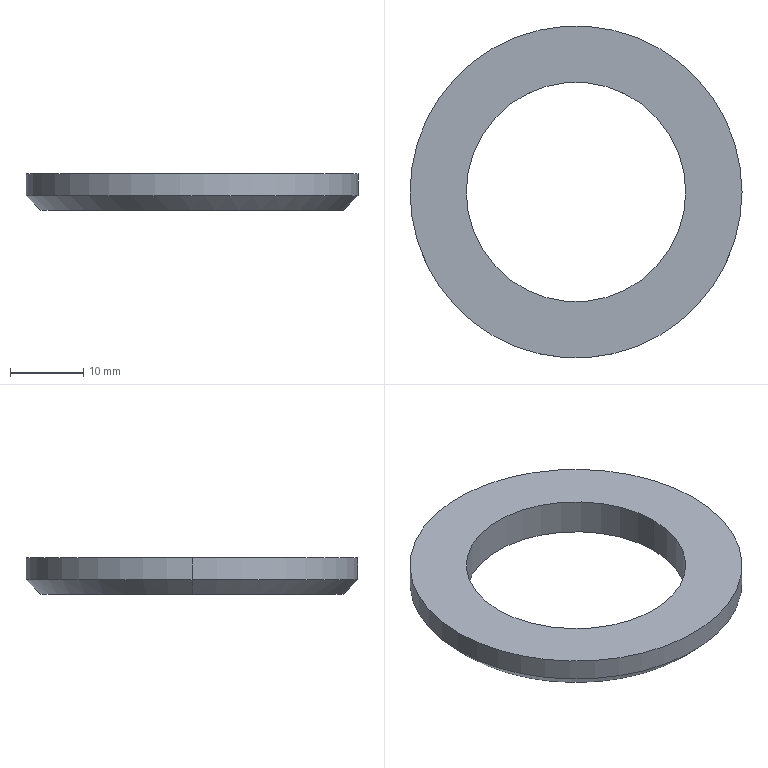Part | SolidWorks | features Chamfer 1, Extrusion 1 | 1 solid | 8 faces | box 45.387 x 45.387 x 5 mm | volume 4279 mm3 | cylinder 4 | cone 2 | plane 2 | commonest cylinder face diameters 30 x2 45.387 x2
STEP:
#1=CARTESIAN_POINT('',(49.306,-13.,0.));
#2=VERTEX_POINT('',#1);
#3=CARTESIAN_POINT('',(90.694,-13.,0.));
#4=VERTEX_POINT('',#3);
#5=CARTESIAN_POINT('',(70.,-13.,0.));
#6=DIRECTION('',(0.,0.,-1.));
#7=DIRECTION('',(1.,0.,0.));
#8=AXIS2_PLACEMENT_3D('',#5,#6,#7);
#9=CIRCLE('',#8,20.694);
#10=EDGE_CURVE('',#2,#4,#9,.T.);
#11=ORIENTED_EDGE('',*,*,#10,.F.);
#12=CARTESIAN_POINT('',(47.306,-13.,2.));
#13=VERTEX_POINT('',#12);
#14=CARTESIAN_POINT('',(47.306,-13.,2.));
#15=DIRECTION('',(-0.7071,0.,0.7071));
#16=VECTOR('',#15,1000.);
#17=LINE('',#14,#16);
#18=EDGE_CURVE('',#2,#13,#17,.T.);
#19=ORIENTED_EDGE('',*,*,#18,.T.);
#20=CARTESIAN_POINT('',(92.694,-13.,2.));
#21=VERTEX_POINT('',#20);
#22=CARTESIAN_POINT('',(70.,-13.,2.));
#23=DIRECTION('',(0.,0.,1.));
#24=DIRECTION('',(1.,0.,0.));
#25=AXIS2_PLACEMENT_3D('',#22,#23,#24);
#26=CIRCLE('',#25,22.694);
#27=EDGE_CURVE('',#21,#13,#26,.T.);
#28=ORIENTED_EDGE('',*,*,#27,.F.);
#29=CARTESIAN_POINT('',(92.694,-13.,2.));
#30=DIRECTION('',(0.7071,0.,0.7071));
#31=VECTOR('',#30,1000.);
#32=LINE('',#29,#31);
#33=EDGE_CURVE('',#4,#21,#32,.T.);
#34=ORIENTED_EDGE('',*,*,#33,.F.);
#35=EDGE_LOOP('',(#11,#19,#28,#34));
#36=FACE_OUTER_BOUND('',#35,.T.);
#37=CARTESIAN_POINT('',(70.,-13.,2.));
#38=DIRECTION('',(0.,0.,1.));
#39=DIRECTION('',(1.,0.,0.));
#40=AXIS2_PLACEMENT_3D('',#37,#38,#39);
#41=CONICAL_SURFACE('',#40,22.694,0.7854);
#42=ADVANCED_FACE('',(#36),#41,.T.);
#43=CARTESIAN_POINT('',(55.,-13.,5.));
#44=VERTEX_POINT('',#43);
#45=CARTESIAN_POINT('',(85.,-13.,5.));
#46=VERTEX_POINT('',#45);
#47=CARTESIAN_POINT('',(70.,-13.,5.));
#48=DIRECTION('',(0.,0.,1.));
#49=DIRECTION('',(1.,0.,0.));
#50=AXIS2_PLACEMENT_3D('',#47,#48,#49);
#51=CIRCLE('',#50,15.);
#52=EDGE_CURVE('',#44,#46,#51,.T.);
#53=ORIENTED_EDGE('',*,*,#52,.T.);
#54=CARTESIAN_POINT('',(85.,-13.,0.));
#55=VERTEX_POINT('',#54);
#56=CARTESIAN_POINT('',(85.,-13.,5.));
#57=DIRECTION('',(0.,0.,-1.));
#58=VECTOR('',#57,1000.);
#59=LINE('',#56,#58);
#60=EDGE_CURVE('',#46,#55,#59,.T.);
#61=ORIENTED_EDGE('',*,*,#60,.T.);
#62=CARTESIAN_POINT('',(55.,-13.,0.));
#63=VERTEX_POINT('',#62);
#64=CARTESIAN_POINT('',(70.,-13.,0.));
#65=DIRECTION('',(0.,0.,1.));
#66=DIRECTION('',(1.,0.,0.));
#67=AXIS2_PLACEMENT_3D('',#64,#65,#66);
#68=CIRCLE('',#67,15.);
#69=EDGE_CURVE('',#63,#55,#68,.T.);
#70=ORIENTED_EDGE('',*,*,#69,.F.);
#71=CARTESIAN_POINT('',(55.,-13.,5.));
#72=DIRECTION('',(0.,0.,-1.));
#73=VECTOR('',#72,1000.);
#74=LINE('',#71,#73);
#75=EDGE_CURVE('',#44,#63,#74,.T.);
#76=ORIENTED_EDGE('',*,*,#75,.F.);
#77=EDGE_LOOP('',(#53,#61,#70,#76));
#78=FACE_OUTER_BOUND('',#77,.T.);
#79=CARTESIAN_POINT('',(70.,-13.,5.));
#80=DIRECTION('',(0.,0.,-1.));
#81=DIRECTION('',(-1.,0.,0.));
#82=AXIS2_PLACEMENT_3D('',#79,#80,#81);
#83=CYLINDRICAL_SURFACE('',#82,15.);
#84=ADVANCED_FACE('',(#78),#83,.F.);
#85=CARTESIAN_POINT('',(92.694,-13.,5.));
#86=VERTEX_POINT('',#85);
#87=CARTESIAN_POINT('',(47.306,-13.,5.));
#88=VERTEX_POINT('',#87);
#89=CARTESIAN_POINT('',(70.,-13.,5.));
#90=DIRECTION('',(0.,0.,1.));
#91=DIRECTION('',(1.,0.,0.));
#92=AXIS2_PLACEMENT_3D('',#89,#90,#91);
#93=CIRCLE('',#92,22.694);
#94=EDGE_CURVE('',#86,#88,#93,.T.);
#95=ORIENTED_EDGE('',*,*,#94,.F.);
#96=CARTESIAN_POINT('',(92.694,-13.,5.));
#97=DIRECTION('',(0.,0.,-1.));
#98=VECTOR('',#97,1000.);
#99=LINE('',#96,#98);
#100=EDGE_CURVE('',#86,#21,#99,.T.);
#101=ORIENTED_EDGE('',*,*,#100,.T.);
#102=ORIENTED_EDGE('',*,*,#27,.T.);
#103=CARTESIAN_POINT('',(47.306,-13.,5.));
#104=DIRECTION('',(0.,0.,-1.));
#105=VECTOR('',#104,1000.);
#106=LINE('',#103,#105);
#107=EDGE_CURVE('',#88,#13,#106,.T.);
#108=ORIENTED_EDGE('',*,*,#107,.F.);
#109=EDGE_LOOP('',(#95,#101,#102,#108));
#110=FACE_OUTER_BOUND('',#109,.T.);
#111=CARTESIAN_POINT('',(70.,-13.,5.));
#112=DIRECTION('',(0.,0.,-1.));
#113=DIRECTION('',(-1.,0.,0.));
#114=AXIS2_PLACEMENT_3D('',#111,#112,#113);
#115=CYLINDRICAL_SURFACE('',#114,22.694);
#116=ADVANCED_FACE('',(#110),#115,.T.);
#117=CARTESIAN_POINT('',(70.,-13.,5.));
#118=DIRECTION('',(0.,0.,1.));
#119=DIRECTION('',(1.,0.,0.));
#120=AXIS2_PLACEMENT_3D('',#117,#118,#119);
#121=CIRCLE('',#120,22.694);
#122=EDGE_CURVE('',#88,#86,#121,.T.);
#123=ORIENTED_EDGE('',*,*,#122,.T.);
#124=ORIENTED_EDGE('',*,*,#94,.T.);
#125=EDGE_LOOP('',(#123,#124));
#126=FACE_OUTER_BOUND('',#125,.T.);
#127=ORIENTED_EDGE('',*,*,#52,.F.);
#128=CARTESIAN_POINT('',(70.,-13.,5.));
#129=DIRECTION('',(0.,0.,1.));
#130=DIRECTION('',(1.,0.,0.));
#131=AXIS2_PLACEMENT_3D('',#128,#129,#130);
#132=CIRCLE('',#131,15.);
#133=EDGE_CURVE('',#46,#44,#132,.T.);
#134=ORIENTED_EDGE('',*,*,#133,.F.);
#135=EDGE_LOOP('',(#127,#134));
#136=FACE_BOUND('',#135,.T.);
#137=CARTESIAN_POINT('',(70.,-13.,5.));
#138=DIRECTION('',(0.,0.,1.));
#139=DIRECTION('',(1.,0.,0.));
#140=AXIS2_PLACEMENT_3D('',#137,#138,#139);
#141=PLANE('',#140);
#142=ADVANCED_FACE('',(#126,#136),#141,.T.);
#143=CARTESIAN_POINT('',(70.,-13.,0.));
#144=DIRECTION('',(0.,0.,-1.));
#145=DIRECTION('',(1.,0.,0.));
#146=AXIS2_PLACEMENT_3D('',#143,#144,#145);
#147=CIRCLE('',#146,20.694);
#148=EDGE_CURVE('',#4,#2,#147,.T.);
#149=ORIENTED_EDGE('',*,*,#148,.T.);
#150=ORIENTED_EDGE('',*,*,#10,.T.);
#151=EDGE_LOOP('',(#149,#150));
#152=FACE_OUTER_BOUND('',#151,.T.);
#153=ORIENTED_EDGE('',*,*,#69,.T.);
#154=CARTESIAN_POINT('',(70.,-13.,0.));
#155=DIRECTION('',(0.,0.,1.));
#156=DIRECTION('',(1.,0.,0.));
#157=AXIS2_PLACEMENT_3D('',#154,#155,#156);
#158=CIRCLE('',#157,15.);
#159=EDGE_CURVE('',#55,#63,#158,.T.);
#160=ORIENTED_EDGE('',*,*,#159,.T.);
#161=EDGE_LOOP('',(#153,#160));
#162=FACE_BOUND('',#161,.T.);
#163=CARTESIAN_POINT('',(70.,-13.,0.));
#164=DIRECTION('',(0.,0.,1.));
#165=DIRECTION('',(1.,0.,0.));
#166=AXIS2_PLACEMENT_3D('',#163,#164,#165);
#167=PLANE('',#166);
#168=ADVANCED_FACE('',(#152,#162),#167,.F.);
#169=ORIENTED_EDGE('',*,*,#100,.F.);
#170=ORIENTED_EDGE('',*,*,#122,.F.);
#171=ORIENTED_EDGE('',*,*,#107,.T.);
#172=CARTESIAN_POINT('',(70.,-13.,2.));
#173=DIRECTION('',(0.,0.,1.));
#174=DIRECTION('',(1.,0.,0.));
#175=AXIS2_PLACEMENT_3D('',#172,#173,#174);
#176=CIRCLE('',#175,22.694);
#177=EDGE_CURVE('',#13,#21,#176,.T.);
#178=ORIENTED_EDGE('',*,*,#177,.T.);
#179=EDGE_LOOP('',(#169,#170,#171,#178));
#180=FACE_OUTER_BOUND('',#179,.T.);
#181=CARTESIAN_POINT('',(70.,-13.,5.));
#182=DIRECTION('',(0.,0.,-1.));
#183=DIRECTION('',(-1.,0.,0.));
#184=AXIS2_PLACEMENT_3D('',#181,#182,#183);
#185=CYLINDRICAL_SURFACE('',#184,22.694);
#186=ADVANCED_FACE('',(#180),#185,.T.);
#187=ORIENTED_EDGE('',*,*,#60,.F.);
#188=ORIENTED_EDGE('',*,*,#133,.T.);
#189=ORIENTED_EDGE('',*,*,#75,.T.);
#190=ORIENTED_EDGE('',*,*,#159,.F.);
#191=EDGE_LOOP('',(#187,#188,#189,#190));
#192=FACE_OUTER_BOUND('',#191,.T.);
#193=CARTESIAN_POINT('',(70.,-13.,5.));
#194=DIRECTION('',(0.,0.,-1.));
#195=DIRECTION('',(-1.,0.,0.));
#196=AXIS2_PLACEMENT_3D('',#193,#194,#195);
#197=CYLINDRICAL_SURFACE('',#196,15.);
#198=ADVANCED_FACE('',(#192),#197,.F.);
#199=ORIENTED_EDGE('',*,*,#18,.F.);
#200=ORIENTED_EDGE('',*,*,#148,.F.);
#201=ORIENTED_EDGE('',*,*,#33,.T.);
#202=ORIENTED_EDGE('',*,*,#177,.F.);
#203=EDGE_LOOP('',(#199,#200,#201,#202));
#204=FACE_OUTER_BOUND('',#203,.T.);
#205=CARTESIAN_POINT('',(70.,-13.,2.));
#206=DIRECTION('',(0.,0.,1.));
#207=DIRECTION('',(1.,0.,0.));
#208=AXIS2_PLACEMENT_3D('',#205,#206,#207);
#209=CONICAL_SURFACE('',#208,22.694,0.7854);
#210=ADVANCED_FACE('',(#204),#209,.T.);
#211=CLOSED_SHELL('',(#42,#84,#116,#142,#168,#186,#198,#210));
#212=MANIFOLD_SOLID_BREP('',#211);
#213=CARTESIAN_POINT('',(0.,0.,0.));
#214=DIRECTION('',(0.,0.,1.));
#215=DIRECTION('',(1.,0.,0.));
#216=AXIS2_PLACEMENT_3D('',#213,#214,#215);
#217=(LENGTH_UNIT()NAMED_UNIT(*)SI_UNIT(.MILLI.,.METRE.));
#218=UNCERTAINTY_MEASURE_WITH_UNIT(LENGTH_MEASURE(0.00001),#217,'','');
#219=(NAMED_UNIT(*)PLANE_ANGLE_UNIT()SI_UNIT($,.RADIAN.));
#220=(NAMED_UNIT(*)SI_UNIT($,.STERADIAN.)SOLID_ANGLE_UNIT());
#221=(GEOMETRIC_REPRESENTATION_CONTEXT(3)GLOBAL_UNCERTAINTY_ASSIGNED_CONTEXT((#218))GLOBAL_UNIT_ASSIGNED_CONTEXT((#217,#219,#220))REPRESENTATION_CONTEXT('',''));
#222=ADVANCED_BREP_SHAPE_REPRESENTATION('',(#212,#216),#221);